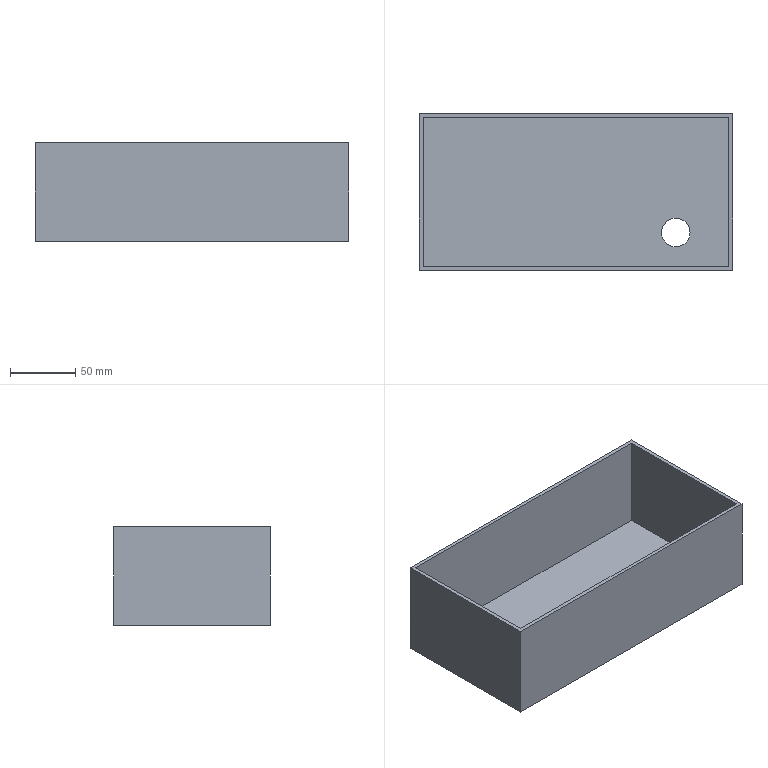Part | STEP file | xiang | 1 solid | 12 faces | box 240 x 120 x 75.5 mm | volume 239250 mm3 | plane 11 | cylinder 1 | commonest cylinder face diameters 22 x1
STEP:
#1=CARTESIAN_POINT('',(0.,0.,0.));
#2=DIRECTION('',(0.,0.,1.));
#3=DIRECTION('',(1.,0.,0.));
#4=AXIS2_PLACEMENT_3D('',#1,#2,#3);
#5=CARTESIAN_POINT('',(65.515,-31.,1.5));
#6=VERTEX_POINT('',#5);
#7=CARTESIAN_POINT('',(76.515,-31.,1.5));
#8=DIRECTION('',(0.,0.,-1.));
#9=DIRECTION('',(-1.,0.,0.));
#10=AXIS2_PLACEMENT_3D('',#7,#8,#9);
#11=CIRCLE('',#10,11.);
#12=CARTESIAN_POINT('',(0.,0.,1.5));
#13=DIRECTION('',(0.,0.,1.));
#14=DIRECTION('',(1.,0.,0.));
#15=AXIS2_PLACEMENT_3D('',#12,#13,#14);
#16=PLANE('',#15);
#17=CARTESIAN_POINT('',(65.515,-31.));
#18=CARTESIAN_POINT('',(65.515,-11.947));
#19=CARTESIAN_POINT('',(82.015,-21.474));
#20=CARTESIAN_POINT('',(98.515,-31.));
#21=CARTESIAN_POINT('',(82.015,-40.526));
#22=CARTESIAN_POINT('',(65.515,-50.053));
#23=CARTESIAN_POINT('',(65.515,-31.));
#24=(BOUNDED_CURVE()B_SPLINE_CURVE(2,(#17,#18,#19,#20,#21,#22,#23),.UNSPECIFIED.,.T.,.F.)B_SPLINE_CURVE_WITH_KNOTS((1,2,2,2,2,1),(-2.094,0.,2.094,4.189,6.283,8.378),.UNSPECIFIED.)CURVE()GEOMETRIC_REPRESENTATION_ITEM()RATIONAL_B_SPLINE_CURVE((1.,0.5,1.,0.5,1.,0.5,1.))REPRESENTATION_ITEM(''));
#25=(GEOMETRIC_REPRESENTATION_CONTEXT(2)PARAMETRIC_REPRESENTATION_CONTEXT()REPRESENTATION_CONTEXT('',''));
#26=DEFINITIONAL_REPRESENTATION('',(#24),#25);
#27=PCURVE('',#16,#26);
#28=CARTESIAN_POINT('',(76.515,-31.,1.5));
#29=DIRECTION('',(0.,0.,-1.));
#30=DIRECTION('',(-1.,0.,0.));
#31=AXIS2_PLACEMENT_3D('',#28,#29,#30);
#32=CYLINDRICAL_SURFACE('',#31,11.);
#33=CARTESIAN_POINT('',(0.,0.));
#34=DIRECTION('',(1.,0.));
#35=VECTOR('',#34,1.);
#36=LINE('',#33,#35);
#37=(GEOMETRIC_REPRESENTATION_CONTEXT(2)PARAMETRIC_REPRESENTATION_CONTEXT()REPRESENTATION_CONTEXT('',''));
#38=DEFINITIONAL_REPRESENTATION('',(#36),#37);
#39=PCURVE('',#32,#38);
#40=SURFACE_CURVE('',#11,(#27,#39),.PCURVE_S1.);
#41=EDGE_CURVE('',#6,#6,#40,.T.);
#42=ORIENTED_EDGE('',*,*,#41,.T.);
#43=EDGE_LOOP('',(#42));
#44=FACE_BOUND('',#43,.T.);
#45=CARTESIAN_POINT('',(117.,-57.,1.5));
#46=VERTEX_POINT('',#45);
#47=CARTESIAN_POINT('',(117.,57.,1.5));
#48=VERTEX_POINT('',#47);
#49=CARTESIAN_POINT('',(117.,60.,1.5));
#50=DIRECTION('',(0.,1.,0.));
#51=VECTOR('',#50,1.);
#52=LINE('',#49,#51);
#53=CARTESIAN_POINT('',(117.,60.));
#54=DIRECTION('',(0.,1.));
#55=VECTOR('',#54,1.);
#56=LINE('',#53,#55);
#57=(GEOMETRIC_REPRESENTATION_CONTEXT(2)PARAMETRIC_REPRESENTATION_CONTEXT()REPRESENTATION_CONTEXT('',''));
#58=DEFINITIONAL_REPRESENTATION('',(#56),#57);
#59=PCURVE('',#16,#58);
#60=CARTESIAN_POINT('',(117.,0.,0.));
#61=DIRECTION('',(-1.,0.,0.));
#62=DIRECTION('',(0.,-1.,0.));
#63=AXIS2_PLACEMENT_3D('',#60,#61,#62);
#64=PLANE('',#63);
#65=CARTESIAN_POINT('',(-60.,1.5));
#66=DIRECTION('',(-1.,0.));
#67=VECTOR('',#66,1.);
#68=LINE('',#65,#67);
#69=(GEOMETRIC_REPRESENTATION_CONTEXT(2)PARAMETRIC_REPRESENTATION_CONTEXT()REPRESENTATION_CONTEXT('',''));
#70=DEFINITIONAL_REPRESENTATION('',(#68),#69);
#71=PCURVE('',#64,#70);
#72=SURFACE_CURVE('',#52,(#59,#71),.PCURVE_S1.);
#73=EDGE_CURVE('',#46,#48,#72,.T.);
#74=ORIENTED_EDGE('',*,*,#73,.T.);
#75=CARTESIAN_POINT('',(-117.,57.,1.5));
#76=VERTEX_POINT('',#75);
#77=CARTESIAN_POINT('',(0.,57.,1.5));
#78=DIRECTION('',(-1.,0.,0.));
#79=VECTOR('',#78,1.);
#80=LINE('',#77,#79);
#81=CARTESIAN_POINT('',(0.,57.));
#82=DIRECTION('',(-1.,0.));
#83=VECTOR('',#82,1.);
#84=LINE('',#81,#83);
#85=(GEOMETRIC_REPRESENTATION_CONTEXT(2)PARAMETRIC_REPRESENTATION_CONTEXT()REPRESENTATION_CONTEXT('',''));
#86=DEFINITIONAL_REPRESENTATION('',(#84),#85);
#87=PCURVE('',#16,#86);
#88=CARTESIAN_POINT('',(0.,57.,0.));
#89=DIRECTION('',(0.,1.,0.));
#90=DIRECTION('',(0.,0.,1.));
#91=AXIS2_PLACEMENT_3D('',#88,#89,#90);
#92=PLANE('',#91);
#93=CARTESIAN_POINT('',(1.5,0.));
#94=DIRECTION('',(0.,-1.));
#95=VECTOR('',#94,1.);
#96=LINE('',#93,#95);
#97=(GEOMETRIC_REPRESENTATION_CONTEXT(2)PARAMETRIC_REPRESENTATION_CONTEXT()REPRESENTATION_CONTEXT('',''));
#98=DEFINITIONAL_REPRESENTATION('',(#96),#97);
#99=PCURVE('',#92,#98);
#100=SURFACE_CURVE('',#80,(#87,#99),.PCURVE_S1.);
#101=EDGE_CURVE('',#48,#76,#100,.T.);
#102=ORIENTED_EDGE('',*,*,#101,.T.);
#103=CARTESIAN_POINT('',(-117.,-57.,1.5));
#104=VERTEX_POINT('',#103);
#105=CARTESIAN_POINT('',(-117.,60.,1.5));
#106=DIRECTION('',(0.,-1.,0.));
#107=VECTOR('',#106,1.);
#108=LINE('',#105,#107);
#109=CARTESIAN_POINT('',(-117.,60.));
#110=DIRECTION('',(0.,-1.));
#111=VECTOR('',#110,1.);
#112=LINE('',#109,#111);
#113=(GEOMETRIC_REPRESENTATION_CONTEXT(2)PARAMETRIC_REPRESENTATION_CONTEXT()REPRESENTATION_CONTEXT('',''));
#114=DEFINITIONAL_REPRESENTATION('',(#112),#113);
#115=PCURVE('',#16,#114);
#116=CARTESIAN_POINT('',(-117.,0.,0.));
#117=DIRECTION('',(-1.,0.,0.));
#118=DIRECTION('',(0.,-1.,0.));
#119=AXIS2_PLACEMENT_3D('',#116,#117,#118);
#120=PLANE('',#119);
#121=CARTESIAN_POINT('',(-60.,1.5));
#122=DIRECTION('',(1.,0.));
#123=VECTOR('',#122,1.);
#124=LINE('',#121,#123);
#125=(GEOMETRIC_REPRESENTATION_CONTEXT(2)PARAMETRIC_REPRESENTATION_CONTEXT()REPRESENTATION_CONTEXT('',''));
#126=DEFINITIONAL_REPRESENTATION('',(#124),#125);
#127=PCURVE('',#120,#126);
#128=SURFACE_CURVE('',#108,(#115,#127),.PCURVE_S1.);
#129=EDGE_CURVE('',#76,#104,#128,.T.);
#130=ORIENTED_EDGE('',*,*,#129,.T.);
#131=CARTESIAN_POINT('',(0.,-57.,1.5));
#132=DIRECTION('',(1.,0.,0.));
#133=VECTOR('',#132,1.);
#134=LINE('',#131,#133);
#135=CARTESIAN_POINT('',(0.,-57.));
#136=DIRECTION('',(1.,0.));
#137=VECTOR('',#136,1.);
#138=LINE('',#135,#137);
#139=(GEOMETRIC_REPRESENTATION_CONTEXT(2)PARAMETRIC_REPRESENTATION_CONTEXT()REPRESENTATION_CONTEXT('',''));
#140=DEFINITIONAL_REPRESENTATION('',(#138),#139);
#141=PCURVE('',#16,#140);
#142=CARTESIAN_POINT('',(0.,-57.,0.));
#143=DIRECTION('',(0.,-1.,0.));
#144=DIRECTION('',(0.,0.,-1.));
#145=AXIS2_PLACEMENT_3D('',#142,#143,#144);
#146=PLANE('',#145);
#147=CARTESIAN_POINT('',(-1.5,0.));
#148=DIRECTION('',(0.,1.));
#149=VECTOR('',#148,1.);
#150=LINE('',#147,#149);
#151=(GEOMETRIC_REPRESENTATION_CONTEXT(2)PARAMETRIC_REPRESENTATION_CONTEXT()REPRESENTATION_CONTEXT('',''));
#152=DEFINITIONAL_REPRESENTATION('',(#150),#151);
#153=PCURVE('',#146,#152);
#154=SURFACE_CURVE('',#134,(#141,#153),.PCURVE_S1.);
#155=EDGE_CURVE('',#104,#46,#154,.T.);
#156=ORIENTED_EDGE('',*,*,#155,.T.);
#157=EDGE_LOOP('',(#74,#102,#130,#156));
#158=FACE_BOUND('',#157,.T.);
#159=ADVANCED_FACE('',(#44,#158),#16,.T.);
#160=CARTESIAN_POINT('',(117.,57.,74.));
#161=VERTEX_POINT('',#160);
#162=CARTESIAN_POINT('',(117.,-57.,74.));
#163=VERTEX_POINT('',#162);
#164=CARTESIAN_POINT('',(117.,60.,74.));
#165=DIRECTION('',(0.,-1.,0.));
#166=VECTOR('',#165,1.);
#167=LINE('',#164,#166);
#168=CARTESIAN_POINT('',(-60.,74.));
#169=DIRECTION('',(1.,0.));
#170=VECTOR('',#169,1.);
#171=LINE('',#168,#170);
#172=(GEOMETRIC_REPRESENTATION_CONTEXT(2)PARAMETRIC_REPRESENTATION_CONTEXT()REPRESENTATION_CONTEXT('',''));
#173=DEFINITIONAL_REPRESENTATION('',(#171),#172);
#174=PCURVE('',#64,#173);
#175=CARTESIAN_POINT('',(117.,60.,74.));
#176=DIRECTION('',(0.,0.,1.));
#177=DIRECTION('',(0.,-1.,0.));
#178=AXIS2_PLACEMENT_3D('',#175,#176,#177);
#179=PLANE('',#178);
#180=CARTESIAN_POINT('',(0.,0.));
#181=DIRECTION('',(1.,0.));
#182=VECTOR('',#181,1.);
#183=LINE('',#180,#182);
#184=(GEOMETRIC_REPRESENTATION_CONTEXT(2)PARAMETRIC_REPRESENTATION_CONTEXT()REPRESENTATION_CONTEXT('',''));
#185=DEFINITIONAL_REPRESENTATION('',(#183),#184);
#186=PCURVE('',#179,#185);
#187=SURFACE_CURVE('',#167,(#174,#186),.PCURVE_S1.);
#188=EDGE_CURVE('',#161,#163,#187,.T.);
#189=ORIENTED_EDGE('',*,*,#188,.F.);
#190=CARTESIAN_POINT('',(117.,57.,0.));
#191=DIRECTION('',(0.,0.,-1.));
#192=VECTOR('',#191,1.);
#193=LINE('',#190,#192);
#194=CARTESIAN_POINT('',(-57.,0.));
#195=DIRECTION('',(0.,-1.));
#196=VECTOR('',#195,1.);
#197=LINE('',#194,#196);
#198=(GEOMETRIC_REPRESENTATION_CONTEXT(2)PARAMETRIC_REPRESENTATION_CONTEXT()REPRESENTATION_CONTEXT('',''));
#199=DEFINITIONAL_REPRESENTATION('',(#197),#198);
#200=PCURVE('',#64,#199);
#201=CARTESIAN_POINT('',(0.,117.));
#202=DIRECTION('',(-1.,0.));
#203=VECTOR('',#202,1.);
#204=LINE('',#201,#203);
#205=(GEOMETRIC_REPRESENTATION_CONTEXT(2)PARAMETRIC_REPRESENTATION_CONTEXT()REPRESENTATION_CONTEXT('',''));
#206=DEFINITIONAL_REPRESENTATION('',(#204),#205);
#207=PCURVE('',#92,#206);
#208=SURFACE_CURVE('',#193,(#200,#207),.PCURVE_S1.);
#209=EDGE_CURVE('',#161,#48,#208,.T.);
#210=ORIENTED_EDGE('',*,*,#209,.T.);
#211=ORIENTED_EDGE('',*,*,#73,.F.);
#212=CARTESIAN_POINT('',(117.,-57.,0.));
#213=DIRECTION('',(0.,0.,1.));
#214=VECTOR('',#213,1.);
#215=LINE('',#212,#214);
#216=CARTESIAN_POINT('',(57.,0.));
#217=DIRECTION('',(0.,1.));
#218=VECTOR('',#217,1.);
#219=LINE('',#216,#218);
#220=(GEOMETRIC_REPRESENTATION_CONTEXT(2)PARAMETRIC_REPRESENTATION_CONTEXT()REPRESENTATION_CONTEXT('',''));
#221=DEFINITIONAL_REPRESENTATION('',(#219),#220);
#222=PCURVE('',#64,#221);
#223=CARTESIAN_POINT('',(0.,117.));
#224=DIRECTION('',(-1.,0.));
#225=VECTOR('',#224,1.);
#226=LINE('',#223,#225);
#227=(GEOMETRIC_REPRESENTATION_CONTEXT(2)PARAMETRIC_REPRESENTATION_CONTEXT()REPRESENTATION_CONTEXT('',''));
#228=DEFINITIONAL_REPRESENTATION('',(#226),#227);
#229=PCURVE('',#146,#228);
#230=SURFACE_CURVE('',#215,(#222,#229),.PCURVE_S1.);
#231=EDGE_CURVE('',#46,#163,#230,.T.);
#232=ORIENTED_EDGE('',*,*,#231,.T.);
#233=EDGE_LOOP('',(#189,#210,#211,#232));
#234=FACE_BOUND('',#233,.T.);
#235=ADVANCED_FACE('',(#234),#64,.T.);
#236=CARTESIAN_POINT('',(-117.,57.,74.));
#237=VERTEX_POINT('',#236);
#238=CARTESIAN_POINT('',(-117.,57.,0.));
#239=DIRECTION('',(0.,0.,-1.));
#240=VECTOR('',#239,1.);
#241=LINE('',#238,#240);
#242=CARTESIAN_POINT('',(-57.,0.));
#243=DIRECTION('',(0.,-1.));
#244=VECTOR('',#243,1.);
#245=LINE('',#242,#244);
#246=(GEOMETRIC_REPRESENTATION_CONTEXT(2)PARAMETRIC_REPRESENTATION_CONTEXT()REPRESENTATION_CONTEXT('',''));
#247=DEFINITIONAL_REPRESENTATION('',(#245),#246);
#248=PCURVE('',#120,#247);
#249=CARTESIAN_POINT('',(0.,-117.));
#250=DIRECTION('',(-1.,0.));
#251=VECTOR('',#250,1.);
#252=LINE('',#249,#251);
#253=(GEOMETRIC_REPRESENTATION_CONTEXT(2)PARAMETRIC_REPRESENTATION_CONTEXT()REPRESENTATION_CONTEXT('',''));
#254=DEFINITIONAL_REPRESENTATION('',(#252),#253);
#255=PCURVE('',#92,#254);
#256=SURFACE_CURVE('',#241,(#248,#255),.PCURVE_S1.);
#257=EDGE_CURVE('',#237,#76,#256,.T.);
#258=ORIENTED_EDGE('',*,*,#257,.F.);
#259=CARTESIAN_POINT('',(-117.,-57.,74.));
#260=VERTEX_POINT('',#259);
#261=CARTESIAN_POINT('',(-117.,60.,74.));
#262=DIRECTION('',(0.,1.,0.));
#263=VECTOR('',#262,1.);
#264=LINE('',#261,#263);
#265=CARTESIAN_POINT('',(-60.,74.));
#266=DIRECTION('',(-1.,0.));
#267=VECTOR('',#266,1.);
#268=LINE('',#265,#267);
#269=(GEOMETRIC_REPRESENTATION_CONTEXT(2)PARAMETRIC_REPRESENTATION_CONTEXT()REPRESENTATION_CONTEXT('',''));
#270=DEFINITIONAL_REPRESENTATION('',(#268),#269);
#271=PCURVE('',#120,#270);
#272=CARTESIAN_POINT('',(0.,-234.));
#273=DIRECTION('',(-1.,0.));
#274=VECTOR('',#273,1.);
#275=LINE('',#272,#274);
#276=(GEOMETRIC_REPRESENTATION_CONTEXT(2)PARAMETRIC_REPRESENTATION_CONTEXT()REPRESENTATION_CONTEXT('',''));
#277=DEFINITIONAL_REPRESENTATION('',(#275),#276);
#278=PCURVE('',#179,#277);
#279=SURFACE_CURVE('',#264,(#271,#278),.PCURVE_S1.);
#280=EDGE_CURVE('',#260,#237,#279,.T.);
#281=ORIENTED_EDGE('',*,*,#280,.F.);
#282=CARTESIAN_POINT('',(-117.,-57.,0.));
#283=DIRECTION('',(0.,0.,1.));
#284=VECTOR('',#283,1.);
#285=LINE('',#282,#284);
#286=CARTESIAN_POINT('',(57.,0.));
#287=DIRECTION('',(0.,1.));
#288=VECTOR('',#287,1.);
#289=LINE('',#286,#288);
#290=(GEOMETRIC_REPRESENTATION_CONTEXT(2)PARAMETRIC_REPRESENTATION_CONTEXT()REPRESENTATION_CONTEXT('',''));
#291=DEFINITIONAL_REPRESENTATION('',(#289),#290);
#292=PCURVE('',#120,#291);
#293=CARTESIAN_POINT('',(0.,-117.));
#294=DIRECTION('',(-1.,0.));
#295=VECTOR('',#294,1.);
#296=LINE('',#293,#295);
#297=(GEOMETRIC_REPRESENTATION_CONTEXT(2)PARAMETRIC_REPRESENTATION_CONTEXT()REPRESENTATION_CONTEXT('',''));
#298=DEFINITIONAL_REPRESENTATION('',(#296),#297);
#299=PCURVE('',#146,#298);
#300=SURFACE_CURVE('',#285,(#292,#299),.PCURVE_S1.);
#301=EDGE_CURVE('',#104,#260,#300,.T.);
#302=ORIENTED_EDGE('',*,*,#301,.F.);
#303=ORIENTED_EDGE('',*,*,#129,.F.);
#304=EDGE_LOOP('',(#258,#281,#302,#303));
#305=FACE_BOUND('',#304,.T.);
#306=ADVANCED_FACE('',(#305),#120,.F.);
#307=CARTESIAN_POINT('',(120.,60.,74.));
#308=VERTEX_POINT('',#307);
#309=CARTESIAN_POINT('',(120.,-60.,74.));
#310=VERTEX_POINT('',#309);
#311=CARTESIAN_POINT('',(120.,60.,74.));
#312=DIRECTION('',(0.,-1.,0.));
#313=VECTOR('',#312,1.);
#314=LINE('',#311,#313);
#315=CARTESIAN_POINT('',(120.,60.,1.5));
#316=DIRECTION('',(-1.,0.,0.));
#317=DIRECTION('',(0.,-1.,0.));
#318=AXIS2_PLACEMENT_3D('',#315,#316,#317);
#319=PLANE('',#318);
#320=CARTESIAN_POINT('',(0.,72.5));
#321=DIRECTION('',(1.,0.));
#322=VECTOR('',#321,1.);
#323=LINE('',#320,#322);
#324=(GEOMETRIC_REPRESENTATION_CONTEXT(2)PARAMETRIC_REPRESENTATION_CONTEXT()REPRESENTATION_CONTEXT('',''));
#325=DEFINITIONAL_REPRESENTATION('',(#323),#324);
#326=PCURVE('',#319,#325);
#327=CARTESIAN_POINT('',(0.,3.));
#328=DIRECTION('',(1.,0.));
#329=VECTOR('',#328,1.);
#330=LINE('',#327,#329);
#331=(GEOMETRIC_REPRESENTATION_CONTEXT(2)PARAMETRIC_REPRESENTATION_CONTEXT()REPRESENTATION_CONTEXT('',''));
#332=DEFINITIONAL_REPRESENTATION('',(#330),#331);
#333=PCURVE('',#179,#332);
#334=SURFACE_CURVE('',#314,(#326,#333),.PCURVE_S1.);
#335=EDGE_CURVE('',#308,#310,#334,.T.);
#336=ORIENTED_EDGE('',*,*,#335,.T.);
#337=CARTESIAN_POINT('',(120.,-60.,-1.5));
#338=VERTEX_POINT('',#337);
#339=CARTESIAN_POINT('',(120.,-60.,1.5));
#340=DIRECTION('',(0.,0.,-1.));
#341=VECTOR('',#340,1.);
#342=LINE('',#339,#341);
#343=CARTESIAN_POINT('',(120.,0.));
#344=DIRECTION('',(0.,-1.));
#345=VECTOR('',#344,1.);
#346=LINE('',#343,#345);
#347=(GEOMETRIC_REPRESENTATION_CONTEXT(2)PARAMETRIC_REPRESENTATION_CONTEXT()REPRESENTATION_CONTEXT('',''));
#348=DEFINITIONAL_REPRESENTATION('',(#346),#347);
#349=PCURVE('',#319,#348);
#350=CARTESIAN_POINT('',(-120.,-60.,1.5));
#351=DIRECTION('',(0.,1.,0.));
#352=DIRECTION('',(0.,0.,1.));
#353=AXIS2_PLACEMENT_3D('',#350,#351,#352);
#354=PLANE('',#353);
#355=CARTESIAN_POINT('',(0.,240.));
#356=DIRECTION('',(-1.,0.));
#357=VECTOR('',#356,1.);
#358=LINE('',#355,#357);
#359=(GEOMETRIC_REPRESENTATION_CONTEXT(2)PARAMETRIC_REPRESENTATION_CONTEXT()REPRESENTATION_CONTEXT('',''));
#360=DEFINITIONAL_REPRESENTATION('',(#358),#359);
#361=PCURVE('',#354,#360);
#362=SURFACE_CURVE('',#342,(#349,#361),.PCURVE_S1.);
#363=EDGE_CURVE('',#310,#338,#362,.T.);
#364=ORIENTED_EDGE('',*,*,#363,.T.);
#365=CARTESIAN_POINT('',(120.,60.,-1.5));
#366=VERTEX_POINT('',#365);
#367=CARTESIAN_POINT('',(120.,60.,-1.5));
#368=DIRECTION('',(0.,1.,0.));
#369=VECTOR('',#368,1.);
#370=LINE('',#367,#369);
#371=CARTESIAN_POINT('',(0.,-3.));
#372=DIRECTION('',(-1.,0.));
#373=VECTOR('',#372,1.);
#374=LINE('',#371,#373);
#375=(GEOMETRIC_REPRESENTATION_CONTEXT(2)PARAMETRIC_REPRESENTATION_CONTEXT()REPRESENTATION_CONTEXT('',''));
#376=DEFINITIONAL_REPRESENTATION('',(#374),#375);
#377=PCURVE('',#319,#376);
#378=CARTESIAN_POINT('',(0.,0.,-1.5));
#379=DIRECTION('',(0.,0.,1.));
#380=DIRECTION('',(1.,0.,0.));
#381=AXIS2_PLACEMENT_3D('',#378,#379,#380);
#382=PLANE('',#381);
#383=CARTESIAN_POINT('',(120.,60.));
#384=DIRECTION('',(0.,1.));
#385=VECTOR('',#384,1.);
#386=LINE('',#383,#385);
#387=(GEOMETRIC_REPRESENTATION_CONTEXT(2)PARAMETRIC_REPRESENTATION_CONTEXT()REPRESENTATION_CONTEXT('',''));
#388=DEFINITIONAL_REPRESENTATION('',(#386),#387);
#389=PCURVE('',#382,#388);
#390=SURFACE_CURVE('',#370,(#377,#389),.PCURVE_S1.);
#391=EDGE_CURVE('',#338,#366,#390,.T.);
#392=ORIENTED_EDGE('',*,*,#391,.T.);
#393=CARTESIAN_POINT('',(120.,60.,1.5));
#394=DIRECTION('',(0.,0.,-1.));
#395=VECTOR('',#394,1.);
#396=LINE('',#393,#395);
#397=CARTESIAN_POINT('',(0.,0.));
#398=DIRECTION('',(0.,-1.));
#399=VECTOR('',#398,1.);
#400=LINE('',#397,#399);
#401=(GEOMETRIC_REPRESENTATION_CONTEXT(2)PARAMETRIC_REPRESENTATION_CONTEXT()REPRESENTATION_CONTEXT('',''));
#402=DEFINITIONAL_REPRESENTATION('',(#400),#401);
#403=PCURVE('',#319,#402);
#404=CARTESIAN_POINT('',(-120.,60.,1.5));
#405=DIRECTION('',(0.,-1.,0.));
#406=DIRECTION('',(0.,0.,-1.));
#407=AXIS2_PLACEMENT_3D('',#404,#405,#406);
#408=PLANE('',#407);
#409=CARTESIAN_POINT('',(0.,240.));
#410=DIRECTION('',(1.,0.));
#411=VECTOR('',#410,1.);
#412=LINE('',#409,#411);
#413=(GEOMETRIC_REPRESENTATION_CONTEXT(2)PARAMETRIC_REPRESENTATION_CONTEXT()REPRESENTATION_CONTEXT('',''));
#414=DEFINITIONAL_REPRESENTATION('',(#412),#413);
#415=PCURVE('',#408,#414);
#416=SURFACE_CURVE('',#396,(#403,#415),.PCURVE_S1.);
#417=EDGE_CURVE('',#308,#366,#416,.T.);
#418=ORIENTED_EDGE('',*,*,#417,.F.);
#419=EDGE_LOOP('',(#336,#364,#392,#418));
#420=FACE_BOUND('',#419,.T.);
#421=ADVANCED_FACE('',(#420),#319,.F.);
#422=CARTESIAN_POINT('',(-120.,60.,74.));
#423=VERTEX_POINT('',#422);
#424=CARTESIAN_POINT('',(-120.,60.,-1.5));
#425=VERTEX_POINT('',#424);
#426=CARTESIAN_POINT('',(-120.,60.,1.5));
#427=DIRECTION('',(0.,0.,-1.));
#428=VECTOR('',#427,1.);
#429=LINE('',#426,#428);
#430=CARTESIAN_POINT('',(0.,0.));
#431=DIRECTION('',(1.,0.));
#432=VECTOR('',#431,1.);
#433=LINE('',#430,#432);
#434=(GEOMETRIC_REPRESENTATION_CONTEXT(2)PARAMETRIC_REPRESENTATION_CONTEXT()REPRESENTATION_CONTEXT('',''));
#435=DEFINITIONAL_REPRESENTATION('',(#433),#434);
#436=PCURVE('',#408,#435);
#437=CARTESIAN_POINT('',(-120.,60.,1.5));
#438=DIRECTION('',(1.,0.,0.));
#439=DIRECTION('',(0.,1.,0.));
#440=AXIS2_PLACEMENT_3D('',#437,#438,#439);
#441=PLANE('',#440);
#442=CARTESIAN_POINT('',(0.,0.));
#443=DIRECTION('',(0.,-1.));
#444=VECTOR('',#443,1.);
#445=LINE('',#442,#444);
#446=(GEOMETRIC_REPRESENTATION_CONTEXT(2)PARAMETRIC_REPRESENTATION_CONTEXT()REPRESENTATION_CONTEXT('',''));
#447=DEFINITIONAL_REPRESENTATION('',(#445),#446);
#448=PCURVE('',#441,#447);
#449=SURFACE_CURVE('',#429,(#436,#448),.PCURVE_S1.);
#450=EDGE_CURVE('',#423,#425,#449,.T.);
#451=ORIENTED_EDGE('',*,*,#450,.F.);
#452=CARTESIAN_POINT('',(117.,60.,74.));
#453=DIRECTION('',(1.,0.,0.));
#454=VECTOR('',#453,1.);
#455=LINE('',#452,#454);
#456=CARTESIAN_POINT('',(-72.5,237.));
#457=DIRECTION('',(0.,1.));
#458=VECTOR('',#457,1.);
#459=LINE('',#456,#458);
#460=(GEOMETRIC_REPRESENTATION_CONTEXT(2)PARAMETRIC_REPRESENTATION_CONTEXT()REPRESENTATION_CONTEXT('',''));
#461=DEFINITIONAL_REPRESENTATION('',(#459),#460);
#462=PCURVE('',#408,#461);
#463=CARTESIAN_POINT('',(0.,0.));
#464=DIRECTION('',(0.,1.));
#465=VECTOR('',#464,1.);
#466=LINE('',#463,#465);
#467=(GEOMETRIC_REPRESENTATION_CONTEXT(2)PARAMETRIC_REPRESENTATION_CONTEXT()REPRESENTATION_CONTEXT('',''));
#468=DEFINITIONAL_REPRESENTATION('',(#466),#467);
#469=PCURVE('',#179,#468);
#470=SURFACE_CURVE('',#455,(#462,#469),.PCURVE_S1.);
#471=EDGE_CURVE('',#423,#308,#470,.T.);
#472=ORIENTED_EDGE('',*,*,#471,.T.);
#473=ORIENTED_EDGE('',*,*,#417,.T.);
#474=CARTESIAN_POINT('',(-120.,60.,-1.5));
#475=DIRECTION('',(-1.,0.,0.));
#476=VECTOR('',#475,1.);
#477=LINE('',#474,#476);
#478=CARTESIAN_POINT('',(3.,0.));
#479=DIRECTION('',(0.,-1.));
#480=VECTOR('',#479,1.);
#481=LINE('',#478,#480);
#482=(GEOMETRIC_REPRESENTATION_CONTEXT(2)PARAMETRIC_REPRESENTATION_CONTEXT()REPRESENTATION_CONTEXT('',''));
#483=DEFINITIONAL_REPRESENTATION('',(#481),#482);
#484=PCURVE('',#408,#483);
#485=CARTESIAN_POINT('',(-120.,60.));
#486=DIRECTION('',(-1.,0.));
#487=VECTOR('',#486,1.);
#488=LINE('',#485,#487);
#489=(GEOMETRIC_REPRESENTATION_CONTEXT(2)PARAMETRIC_REPRESENTATION_CONTEXT()REPRESENTATION_CONTEXT('',''));
#490=DEFINITIONAL_REPRESENTATION('',(#488),#489);
#491=PCURVE('',#382,#490);
#492=SURFACE_CURVE('',#477,(#484,#491),.PCURVE_S1.);
#493=EDGE_CURVE('',#366,#425,#492,.T.);
#494=ORIENTED_EDGE('',*,*,#493,.T.);
#495=EDGE_LOOP('',(#451,#472,#473,#494));
#496=FACE_BOUND('',#495,.T.);
#497=ADVANCED_FACE('',(#496),#408,.F.);
#498=CARTESIAN_POINT('',(-120.,-60.,-1.5));
#499=VERTEX_POINT('',#498);
#500=CARTESIAN_POINT('',(-120.,60.,-1.5));
#501=DIRECTION('',(0.,-1.,0.));
#502=VECTOR('',#501,1.);
#503=LINE('',#500,#502);
#504=CARTESIAN_POINT('',(0.,-3.));
#505=DIRECTION('',(-1.,0.));
#506=VECTOR('',#505,1.);
#507=LINE('',#504,#506);
#508=(GEOMETRIC_REPRESENTATION_CONTEXT(2)PARAMETRIC_REPRESENTATION_CONTEXT()REPRESENTATION_CONTEXT('',''));
#509=DEFINITIONAL_REPRESENTATION('',(#507),#508);
#510=PCURVE('',#441,#509);
#511=CARTESIAN_POINT('',(-120.,60.));
#512=DIRECTION('',(0.,-1.));
#513=VECTOR('',#512,1.);
#514=LINE('',#511,#513);
#515=(GEOMETRIC_REPRESENTATION_CONTEXT(2)PARAMETRIC_REPRESENTATION_CONTEXT()REPRESENTATION_CONTEXT('',''));
#516=DEFINITIONAL_REPRESENTATION('',(#514),#515);
#517=PCURVE('',#382,#516);
#518=SURFACE_CURVE('',#503,(#510,#517),.PCURVE_S1.);
#519=EDGE_CURVE('',#425,#499,#518,.T.);
#520=ORIENTED_EDGE('',*,*,#519,.T.);
#521=CARTESIAN_POINT('',(-120.,-60.,74.));
#522=VERTEX_POINT('',#521);
#523=CARTESIAN_POINT('',(-120.,-60.,1.5));
#524=DIRECTION('',(0.,0.,-1.));
#525=VECTOR('',#524,1.);
#526=LINE('',#523,#525);
#527=CARTESIAN_POINT('',(-120.,0.));
#528=DIRECTION('',(0.,-1.));
#529=VECTOR('',#528,1.);
#530=LINE('',#527,#529);
#531=(GEOMETRIC_REPRESENTATION_CONTEXT(2)PARAMETRIC_REPRESENTATION_CONTEXT()REPRESENTATION_CONTEXT('',''));
#532=DEFINITIONAL_REPRESENTATION('',(#530),#531);
#533=PCURVE('',#441,#532);
#534=CARTESIAN_POINT('',(0.,0.));
#535=DIRECTION('',(-1.,0.));
#536=VECTOR('',#535,1.);
#537=LINE('',#534,#536);
#538=(GEOMETRIC_REPRESENTATION_CONTEXT(2)PARAMETRIC_REPRESENTATION_CONTEXT()REPRESENTATION_CONTEXT('',''));
#539=DEFINITIONAL_REPRESENTATION('',(#537),#538);
#540=PCURVE('',#354,#539);
#541=SURFACE_CURVE('',#526,(#533,#540),.PCURVE_S1.);
#542=EDGE_CURVE('',#522,#499,#541,.T.);
#543=ORIENTED_EDGE('',*,*,#542,.F.);
#544=CARTESIAN_POINT('',(-120.,60.,74.));
#545=DIRECTION('',(0.,1.,0.));
#546=VECTOR('',#545,1.);
#547=LINE('',#544,#546);
#548=CARTESIAN_POINT('',(0.,72.5));
#549=DIRECTION('',(1.,0.));
#550=VECTOR('',#549,1.);
#551=LINE('',#548,#550);
#552=(GEOMETRIC_REPRESENTATION_CONTEXT(2)PARAMETRIC_REPRESENTATION_CONTEXT()REPRESENTATION_CONTEXT('',''));
#553=DEFINITIONAL_REPRESENTATION('',(#551),#552);
#554=PCURVE('',#441,#553);
#555=CARTESIAN_POINT('',(0.,-237.));
#556=DIRECTION('',(-1.,0.));
#557=VECTOR('',#556,1.);
#558=LINE('',#555,#557);
#559=(GEOMETRIC_REPRESENTATION_CONTEXT(2)PARAMETRIC_REPRESENTATION_CONTEXT()REPRESENTATION_CONTEXT('',''));
#560=DEFINITIONAL_REPRESENTATION('',(#558),#559);
#561=PCURVE('',#179,#560);
#562=SURFACE_CURVE('',#547,(#554,#561),.PCURVE_S1.);
#563=EDGE_CURVE('',#522,#423,#562,.T.);
#564=ORIENTED_EDGE('',*,*,#563,.T.);
#565=ORIENTED_EDGE('',*,*,#450,.T.);
#566=EDGE_LOOP('',(#520,#543,#564,#565));
#567=FACE_BOUND('',#566,.T.);
#568=ADVANCED_FACE('',(#567),#441,.F.);
#569=CARTESIAN_POINT('',(-120.,-60.,-1.5));
#570=DIRECTION('',(1.,0.,0.));
#571=VECTOR('',#570,1.);
#572=LINE('',#569,#571);
#573=CARTESIAN_POINT('',(-3.,0.));
#574=DIRECTION('',(0.,1.));
#575=VECTOR('',#574,1.);
#576=LINE('',#573,#575);
#577=(GEOMETRIC_REPRESENTATION_CONTEXT(2)PARAMETRIC_REPRESENTATION_CONTEXT()REPRESENTATION_CONTEXT('',''));
#578=DEFINITIONAL_REPRESENTATION('',(#576),#577);
#579=PCURVE('',#354,#578);
#580=CARTESIAN_POINT('',(-120.,-60.));
#581=DIRECTION('',(1.,0.));
#582=VECTOR('',#581,1.);
#583=LINE('',#580,#582);
#584=(GEOMETRIC_REPRESENTATION_CONTEXT(2)PARAMETRIC_REPRESENTATION_CONTEXT()REPRESENTATION_CONTEXT('',''));
#585=DEFINITIONAL_REPRESENTATION('',(#583),#584);
#586=PCURVE('',#382,#585);
#587=SURFACE_CURVE('',#572,(#579,#586),.PCURVE_S1.);
#588=EDGE_CURVE('',#499,#338,#587,.T.);
#589=ORIENTED_EDGE('',*,*,#588,.T.);
#590=ORIENTED_EDGE('',*,*,#363,.F.);
#591=CARTESIAN_POINT('',(117.,-60.,74.));
#592=DIRECTION('',(1.,0.,0.));
#593=VECTOR('',#592,1.);
#594=LINE('',#591,#593);
#595=CARTESIAN_POINT('',(72.5,237.));
#596=DIRECTION('',(0.,1.));
#597=VECTOR('',#596,1.);
#598=LINE('',#595,#597);
#599=(GEOMETRIC_REPRESENTATION_CONTEXT(2)PARAMETRIC_REPRESENTATION_CONTEXT()REPRESENTATION_CONTEXT('',''));
#600=DEFINITIONAL_REPRESENTATION('',(#598),#599);
#601=PCURVE('',#354,#600);
#602=CARTESIAN_POINT('',(120.,0.));
#603=DIRECTION('',(0.,1.));
#604=VECTOR('',#603,1.);
#605=LINE('',#602,#604);
#606=(GEOMETRIC_REPRESENTATION_CONTEXT(2)PARAMETRIC_REPRESENTATION_CONTEXT()REPRESENTATION_CONTEXT('',''));
#607=DEFINITIONAL_REPRESENTATION('',(#605),#606);
#608=PCURVE('',#179,#607);
#609=SURFACE_CURVE('',#594,(#601,#608),.PCURVE_S1.);
#610=EDGE_CURVE('',#522,#310,#609,.T.);
#611=ORIENTED_EDGE('',*,*,#610,.F.);
#612=ORIENTED_EDGE('',*,*,#542,.T.);
#613=EDGE_LOOP('',(#589,#590,#611,#612));
#614=FACE_BOUND('',#613,.T.);
#615=ADVANCED_FACE('',(#614),#354,.F.);
#616=CARTESIAN_POINT('',(65.515,-31.,-1.5));
#617=VERTEX_POINT('',#616);
#618=CARTESIAN_POINT('',(76.515,-31.,-1.5));
#619=DIRECTION('',(0.,0.,-1.));
#620=DIRECTION('',(-1.,0.,0.));
#621=AXIS2_PLACEMENT_3D('',#618,#619,#620);
#622=CIRCLE('',#621,11.);
#623=CARTESIAN_POINT('',(65.515,-31.));
#624=CARTESIAN_POINT('',(65.515,-11.947));
#625=CARTESIAN_POINT('',(82.015,-21.474));
#626=CARTESIAN_POINT('',(98.515,-31.));
#627=CARTESIAN_POINT('',(82.015,-40.526));
#628=CARTESIAN_POINT('',(65.515,-50.053));
#629=CARTESIAN_POINT('',(65.515,-31.));
#630=(BOUNDED_CURVE()B_SPLINE_CURVE(2,(#623,#624,#625,#626,#627,#628,#629),.UNSPECIFIED.,.T.,.F.)B_SPLINE_CURVE_WITH_KNOTS((1,2,2,2,2,1),(-2.094,0.,2.094,4.189,6.283,8.378),.UNSPECIFIED.)CURVE()GEOMETRIC_REPRESENTATION_ITEM()RATIONAL_B_SPLINE_CURVE((1.,0.5,1.,0.5,1.,0.5,1.))REPRESENTATION_ITEM(''));
#631=(GEOMETRIC_REPRESENTATION_CONTEXT(2)PARAMETRIC_REPRESENTATION_CONTEXT()REPRESENTATION_CONTEXT('',''));
#632=DEFINITIONAL_REPRESENTATION('',(#630),#631);
#633=PCURVE('',#382,#632);
#634=CARTESIAN_POINT('',(0.,3.));
#635=DIRECTION('',(1.,0.));
#636=VECTOR('',#635,1.);
#637=LINE('',#634,#636);
#638=(GEOMETRIC_REPRESENTATION_CONTEXT(2)PARAMETRIC_REPRESENTATION_CONTEXT()REPRESENTATION_CONTEXT('',''));
#639=DEFINITIONAL_REPRESENTATION('',(#637),#638);
#640=PCURVE('',#32,#639);
#641=SURFACE_CURVE('',#622,(#633,#640),.PCURVE_S1.);
#642=EDGE_CURVE('',#617,#617,#641,.T.);
#643=ORIENTED_EDGE('',*,*,#642,.F.);
#644=EDGE_LOOP('',(#643));
#645=FACE_BOUND('',#644,.T.);
#646=ORIENTED_EDGE('',*,*,#493,.F.);
#647=ORIENTED_EDGE('',*,*,#391,.F.);
#648=ORIENTED_EDGE('',*,*,#588,.F.);
#649=ORIENTED_EDGE('',*,*,#519,.F.);
#650=EDGE_LOOP('',(#646,#647,#648,#649));
#651=FACE_BOUND('',#650,.T.);
#652=ADVANCED_FACE('',(#645,#651),#382,.F.);
#653=CARTESIAN_POINT('',(-120.,57.,74.));
#654=DIRECTION('',(1.,0.,0.));
#655=VECTOR('',#654,1.);
#656=LINE('',#653,#655);
#657=CARTESIAN_POINT('',(3.,-237.));
#658=DIRECTION('',(0.,1.));
#659=VECTOR('',#658,1.);
#660=LINE('',#657,#659);
#661=(GEOMETRIC_REPRESENTATION_CONTEXT(2)PARAMETRIC_REPRESENTATION_CONTEXT()REPRESENTATION_CONTEXT('',''));
#662=DEFINITIONAL_REPRESENTATION('',(#660),#661);
#663=PCURVE('',#179,#662);
#664=CARTESIAN_POINT('',(74.,-120.));
#665=DIRECTION('',(0.,1.));
#666=VECTOR('',#665,1.);
#667=LINE('',#664,#666);
#668=(GEOMETRIC_REPRESENTATION_CONTEXT(2)PARAMETRIC_REPRESENTATION_CONTEXT()REPRESENTATION_CONTEXT('',''));
#669=DEFINITIONAL_REPRESENTATION('',(#667),#668);
#670=PCURVE('',#92,#669);
#671=SURFACE_CURVE('',#656,(#663,#670),.PCURVE_S1.);
#672=EDGE_CURVE('',#237,#161,#671,.T.);
#673=ORIENTED_EDGE('',*,*,#672,.T.);
#674=ORIENTED_EDGE('',*,*,#188,.T.);
#675=CARTESIAN_POINT('',(-120.,-57.,74.));
#676=DIRECTION('',(-1.,0.,0.));
#677=VECTOR('',#676,1.);
#678=LINE('',#675,#677);
#679=CARTESIAN_POINT('',(117.,-237.));
#680=DIRECTION('',(0.,-1.));
#681=VECTOR('',#680,1.);
#682=LINE('',#679,#681);
#683=(GEOMETRIC_REPRESENTATION_CONTEXT(2)PARAMETRIC_REPRESENTATION_CONTEXT()REPRESENTATION_CONTEXT('',''));
#684=DEFINITIONAL_REPRESENTATION('',(#682),#683);
#685=PCURVE('',#179,#684);
#686=CARTESIAN_POINT('',(-74.,-120.));
#687=DIRECTION('',(0.,-1.));
#688=VECTOR('',#687,1.);
#689=LINE('',#686,#688);
#690=(GEOMETRIC_REPRESENTATION_CONTEXT(2)PARAMETRIC_REPRESENTATION_CONTEXT()REPRESENTATION_CONTEXT('',''));
#691=DEFINITIONAL_REPRESENTATION('',(#689),#690);
#692=PCURVE('',#146,#691);
#693=SURFACE_CURVE('',#678,(#685,#692),.PCURVE_S1.);
#694=EDGE_CURVE('',#163,#260,#693,.T.);
#695=ORIENTED_EDGE('',*,*,#694,.T.);
#696=ORIENTED_EDGE('',*,*,#280,.T.);
#697=EDGE_LOOP('',(#673,#674,#695,#696));
#698=FACE_BOUND('',#697,.T.);
#699=ORIENTED_EDGE('',*,*,#471,.F.);
#700=ORIENTED_EDGE('',*,*,#563,.F.);
#701=ORIENTED_EDGE('',*,*,#610,.T.);
#702=ORIENTED_EDGE('',*,*,#335,.F.);
#703=EDGE_LOOP('',(#699,#700,#701,#702));
#704=FACE_BOUND('',#703,.T.);
#705=ADVANCED_FACE('',(#698,#704),#179,.T.);
#706=ORIENTED_EDGE('',*,*,#231,.F.);
#707=ORIENTED_EDGE('',*,*,#155,.F.);
#708=ORIENTED_EDGE('',*,*,#301,.T.);
#709=ORIENTED_EDGE('',*,*,#694,.F.);
#710=EDGE_LOOP('',(#706,#707,#708,#709));
#711=FACE_BOUND('',#710,.T.);
#712=ADVANCED_FACE('',(#711),#146,.F.);
#713=ORIENTED_EDGE('',*,*,#209,.F.);
#714=ORIENTED_EDGE('',*,*,#672,.F.);
#715=ORIENTED_EDGE('',*,*,#257,.T.);
#716=ORIENTED_EDGE('',*,*,#101,.F.);
#717=EDGE_LOOP('',(#713,#714,#715,#716));
#718=FACE_BOUND('',#717,.T.);
#719=ADVANCED_FACE('',(#718),#92,.F.);
#720=ORIENTED_EDGE('',*,*,#41,.T.);
#721=CARTESIAN_POINT('',(65.515,-31.,1.5));
#722=CARTESIAN_POINT('',(65.515,-31.,-1.5));
#723=B_SPLINE_CURVE_WITH_KNOTS('',1,(#721,#722),.UNSPECIFIED.,.F.,.F.,(2,2),(0.,3.),.PIECEWISE_BEZIER_KNOTS.);
#724=CARTESIAN_POINT('',(6.283,0.));
#725=DIRECTION('',(0.,1.));
#726=VECTOR('',#725,1.);
#727=LINE('',#724,#726);
#728=(GEOMETRIC_REPRESENTATION_CONTEXT(2)PARAMETRIC_REPRESENTATION_CONTEXT()REPRESENTATION_CONTEXT('',''));
#729=DEFINITIONAL_REPRESENTATION('',(#727),#728);
#730=PCURVE('',#32,#729);
#731=CARTESIAN_POINT('',(0.,0.));
#732=DIRECTION('',(0.,1.));
#733=VECTOR('',#732,1.);
#734=LINE('',#731,#733);
#735=(GEOMETRIC_REPRESENTATION_CONTEXT(2)PARAMETRIC_REPRESENTATION_CONTEXT()REPRESENTATION_CONTEXT('',''));
#736=DEFINITIONAL_REPRESENTATION('',(#734),#735);
#737=PCURVE('',#32,#736);
#738=SEAM_CURVE('',#723,(#730,#737),.PCURVE_S1.);
#739=EDGE_CURVE('',#6,#617,#738,.T.);
#740=ORIENTED_EDGE('',*,*,#739,.T.);
#741=ORIENTED_EDGE('',*,*,#642,.F.);
#742=ORIENTED_EDGE('',*,*,#739,.F.);
#743=EDGE_LOOP('',(#720,#740,#741,#742));
#744=FACE_BOUND('',#743,.F.);
#745=ADVANCED_FACE('',(#744),#32,.F.);
#746=CLOSED_SHELL('',(#159,#235,#306,#421,#497,#568,#615,#652,#705,#712,#719,#745));
#747=MANIFOLD_SOLID_BREP('',#746);
#748=(LENGTH_UNIT()NAMED_UNIT(*)SI_UNIT(.MILLI.,.METRE.));
#749=UNCERTAINTY_MEASURE_WITH_UNIT(LENGTH_MEASURE(0.000001),#748,'','');
#750=(NAMED_UNIT(*)PLANE_ANGLE_UNIT()SI_UNIT($,.RADIAN.));
#751=(NAMED_UNIT(*)SI_UNIT($,.STERADIAN.)SOLID_ANGLE_UNIT());
#752=(GEOMETRIC_REPRESENTATION_CONTEXT(3)GLOBAL_UNCERTAINTY_ASSIGNED_CONTEXT((#749))GLOBAL_UNIT_ASSIGNED_CONTEXT((#748,#750,#751))REPRESENTATION_CONTEXT('',''));
#753=ADVANCED_BREP_SHAPE_REPRESENTATION('',(#4,#747),#752);